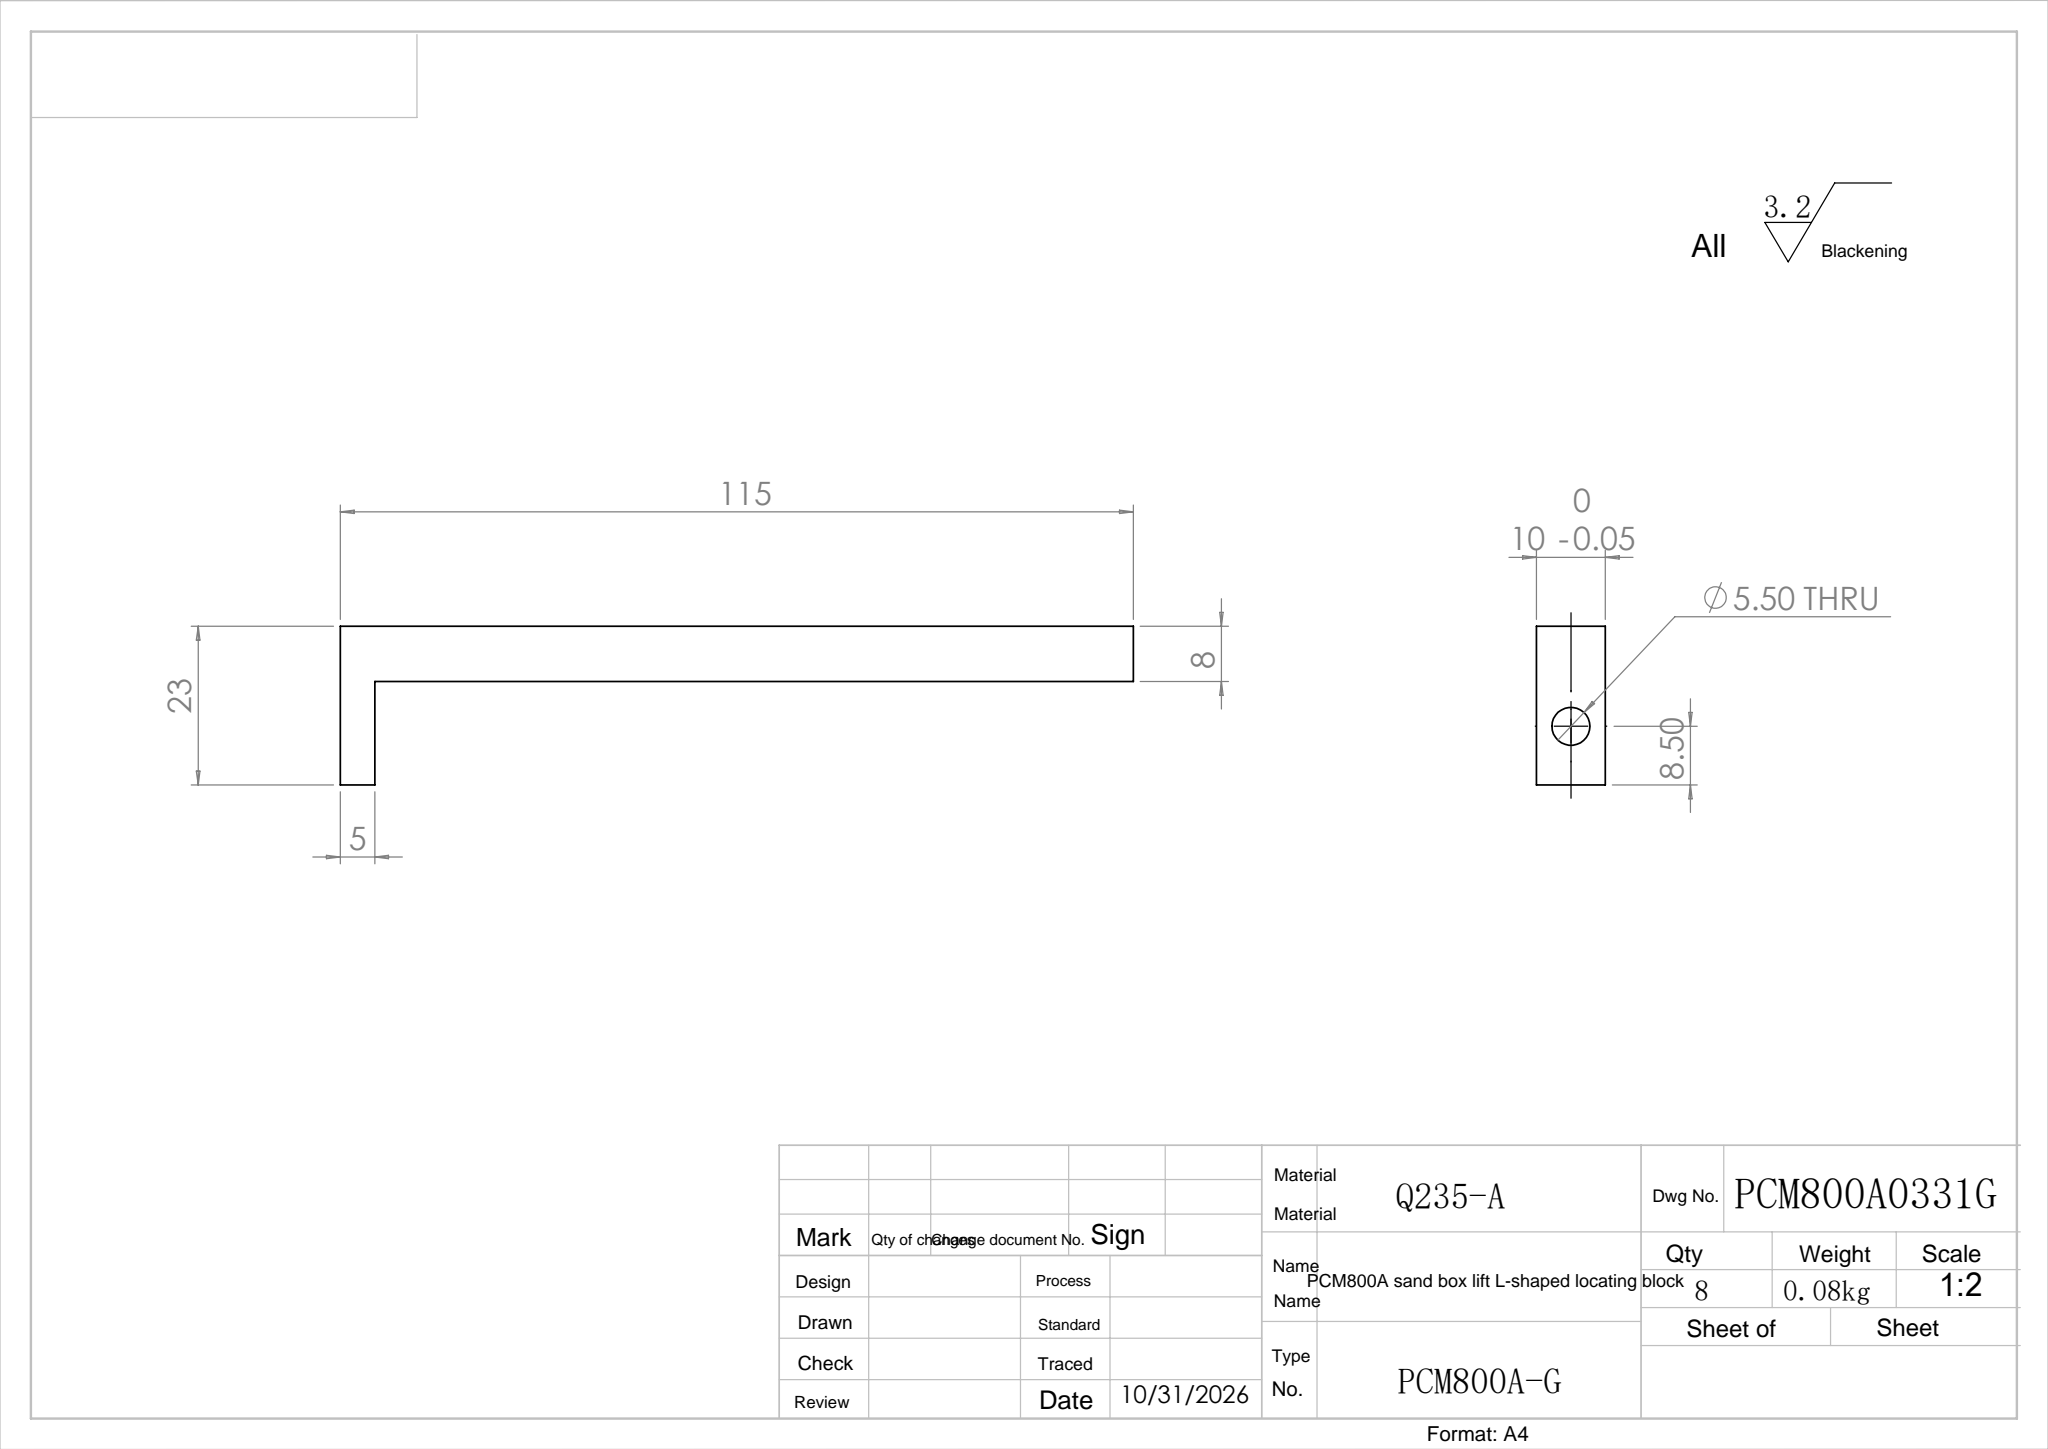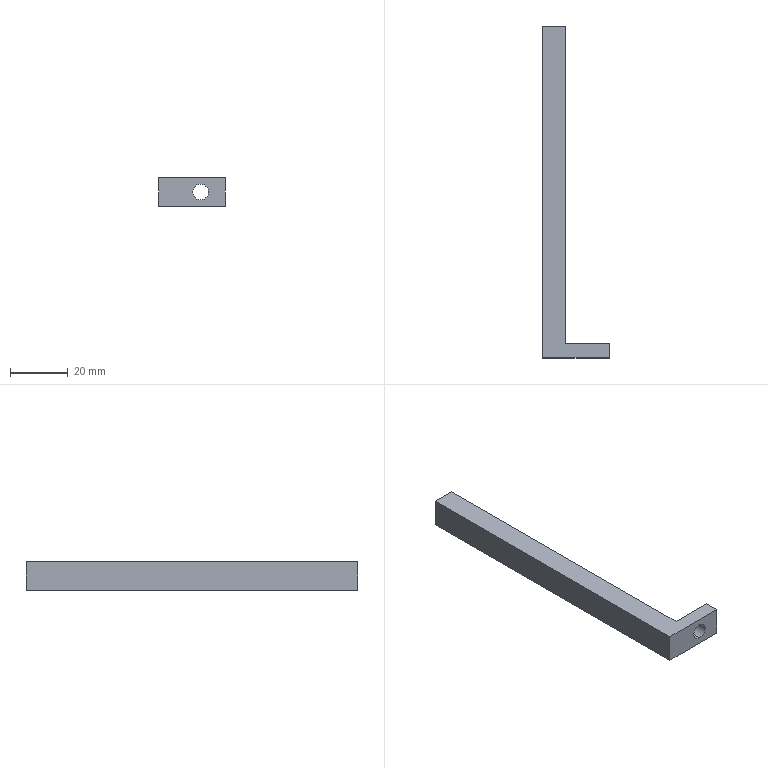Part | SolidWorks | features Extrusion 1, ICE 1 | 1 solid | 10 faces | box 23 x 115 x 10 mm | volume 9831 mm3 | plane 8 | cylinder 2 | commonest cylinder face diameters 5.5 x2
STEP:
#1=CARTESIAN_POINT('',(6.5,-110.,2.25));
#2=VERTEX_POINT('',#1);
#3=CARTESIAN_POINT('',(6.5,-110.,7.75));
#4=VERTEX_POINT('',#3);
#5=CARTESIAN_POINT('',(6.5,-110.,5.));
#6=DIRECTION('',(0.,1.,0.));
#7=DIRECTION('',(0.,0.,1.));
#8=AXIS2_PLACEMENT_3D('',#5,#6,#7);
#9=CIRCLE('',#8,2.75);
#10=EDGE_CURVE('',#2,#4,#9,.T.);
#11=ORIENTED_EDGE('',*,*,#10,.T.);
#12=CARTESIAN_POINT('',(6.5,-115.,7.75));
#13=VERTEX_POINT('',#12);
#14=CARTESIAN_POINT('',(6.5,0.,7.75));
#15=DIRECTION('',(0.,-1.,0.));
#16=VECTOR('',#15,1000.);
#17=LINE('',#14,#16);
#18=EDGE_CURVE('',#4,#13,#17,.T.);
#19=ORIENTED_EDGE('',*,*,#18,.T.);
#20=CARTESIAN_POINT('',(6.5,-115.,2.25));
#21=VERTEX_POINT('',#20);
#22=CARTESIAN_POINT('',(6.5,-115.,5.));
#23=DIRECTION('',(0.,-1.,0.));
#24=DIRECTION('',(0.,0.,-1.));
#25=AXIS2_PLACEMENT_3D('',#22,#23,#24);
#26=CIRCLE('',#25,2.75);
#27=EDGE_CURVE('',#13,#21,#26,.T.);
#28=ORIENTED_EDGE('',*,*,#27,.T.);
#29=CARTESIAN_POINT('',(6.5,0.,2.25));
#30=DIRECTION('',(0.,-1.,0.));
#31=VECTOR('',#30,1000.);
#32=LINE('',#29,#31);
#33=EDGE_CURVE('',#2,#21,#32,.T.);
#34=ORIENTED_EDGE('',*,*,#33,.F.);
#35=EDGE_LOOP('',(#11,#19,#28,#34));
#36=FACE_OUTER_BOUND('',#35,.T.);
#37=CARTESIAN_POINT('',(6.5,0.,5.));
#38=DIRECTION('',(0.,-1.,0.));
#39=DIRECTION('',(0.,0.,-1.));
#40=AXIS2_PLACEMENT_3D('',#37,#38,#39);
#41=CYLINDRICAL_SURFACE('',#40,2.75);
#42=ADVANCED_FACE('',(#36),#41,.F.);
#43=CARTESIAN_POINT('',(6.5,-115.,5.));
#44=DIRECTION('',(0.,-1.,0.));
#45=DIRECTION('',(0.,0.,-1.));
#46=AXIS2_PLACEMENT_3D('',#43,#44,#45);
#47=CIRCLE('',#46,2.75);
#48=EDGE_CURVE('',#21,#13,#47,.T.);
#49=ORIENTED_EDGE('',*,*,#48,.F.);
#50=ORIENTED_EDGE('',*,*,#27,.F.);
#51=EDGE_LOOP('',(#49,#50));
#52=FACE_BOUND('',#51,.T.);
#53=CARTESIAN_POINT('',(15.,-115.,0.));
#54=VERTEX_POINT('',#53);
#55=CARTESIAN_POINT('',(-8.,-115.,0.));
#56=VERTEX_POINT('',#55);
#57=CARTESIAN_POINT('',(3.5,-115.,0.));
#58=DIRECTION('',(-1.,0.,0.));
#59=VECTOR('',#58,1000.);
#60=LINE('',#57,#59);
#61=EDGE_CURVE('',#54,#56,#60,.T.);
#62=ORIENTED_EDGE('',*,*,#61,.F.);
#63=CARTESIAN_POINT('',(15.,-115.,10.));
#64=VERTEX_POINT('',#63);
#65=CARTESIAN_POINT('',(15.,-115.,10.));
#66=DIRECTION('',(0.,0.,-1.));
#67=VECTOR('',#66,1000.);
#68=LINE('',#65,#67);
#69=EDGE_CURVE('',#64,#54,#68,.T.);
#70=ORIENTED_EDGE('',*,*,#69,.F.);
#71=CARTESIAN_POINT('',(-8.,-115.,10.));
#72=VERTEX_POINT('',#71);
#73=CARTESIAN_POINT('',(3.5,-115.,10.));
#74=DIRECTION('',(-1.,0.,0.));
#75=VECTOR('',#74,1000.);
#76=LINE('',#73,#75);
#77=EDGE_CURVE('',#64,#72,#76,.T.);
#78=ORIENTED_EDGE('',*,*,#77,.T.);
#79=CARTESIAN_POINT('',(-8.,-115.,10.));
#80=DIRECTION('',(0.,0.,-1.));
#81=VECTOR('',#80,1000.);
#82=LINE('',#79,#81);
#83=EDGE_CURVE('',#72,#56,#82,.T.);
#84=ORIENTED_EDGE('',*,*,#83,.T.);
#85=EDGE_LOOP('',(#62,#70,#78,#84));
#86=FACE_OUTER_BOUND('',#85,.T.);
#87=CARTESIAN_POINT('',(3.5,-115.,10.));
#88=DIRECTION('',(0.,-1.,0.));
#89=DIRECTION('',(0.,0.,-1.));
#90=AXIS2_PLACEMENT_3D('',#87,#88,#89);
#91=PLANE('',#90);
#92=ADVANCED_FACE('',(#52,#86),#91,.T.);
#93=CARTESIAN_POINT('',(15.,-110.,0.));
#94=VERTEX_POINT('',#93);
#95=CARTESIAN_POINT('',(15.,-148.862,0.));
#96=DIRECTION('',(0.,-1.,0.));
#97=VECTOR('',#96,1000.);
#98=LINE('',#95,#97);
#99=EDGE_CURVE('',#94,#54,#98,.T.);
#100=ORIENTED_EDGE('',*,*,#99,.F.);
#101=CARTESIAN_POINT('',(15.,-110.,10.));
#102=VERTEX_POINT('',#101);
#103=CARTESIAN_POINT('',(15.,-110.,10.));
#104=DIRECTION('',(0.,0.,-1.));
#105=VECTOR('',#104,1000.);
#106=LINE('',#103,#105);
#107=EDGE_CURVE('',#102,#94,#106,.T.);
#108=ORIENTED_EDGE('',*,*,#107,.F.);
#109=CARTESIAN_POINT('',(15.,-148.862,10.));
#110=DIRECTION('',(0.,-1.,0.));
#111=VECTOR('',#110,1000.);
#112=LINE('',#109,#111);
#113=EDGE_CURVE('',#102,#64,#112,.T.);
#114=ORIENTED_EDGE('',*,*,#113,.T.);
#115=ORIENTED_EDGE('',*,*,#69,.T.);
#116=EDGE_LOOP('',(#100,#108,#114,#115));
#117=FACE_OUTER_BOUND('',#116,.T.);
#118=CARTESIAN_POINT('',(15.,-148.862,10.));
#119=DIRECTION('',(1.,0.,0.));
#120=DIRECTION('',(0.,0.,-1.));
#121=AXIS2_PLACEMENT_3D('',#118,#119,#120);
#122=PLANE('',#121);
#123=ADVANCED_FACE('',(#117),#122,.T.);
#124=ORIENTED_EDGE('',*,*,#10,.F.);
#125=CARTESIAN_POINT('',(6.5,-110.,5.));
#126=DIRECTION('',(0.,1.,0.));
#127=DIRECTION('',(0.,0.,1.));
#128=AXIS2_PLACEMENT_3D('',#125,#126,#127);
#129=CIRCLE('',#128,2.75);
#130=EDGE_CURVE('',#4,#2,#129,.T.);
#131=ORIENTED_EDGE('',*,*,#130,.F.);
#132=EDGE_LOOP('',(#124,#131));
#133=FACE_BOUND('',#132,.T.);
#134=CARTESIAN_POINT('',(0.,-110.,0.));
#135=VERTEX_POINT('',#134);
#136=CARTESIAN_POINT('',(3.5,-110.,0.));
#137=DIRECTION('',(1.,0.,0.));
#138=VECTOR('',#137,1000.);
#139=LINE('',#136,#138);
#140=EDGE_CURVE('',#135,#94,#139,.T.);
#141=ORIENTED_EDGE('',*,*,#140,.F.);
#142=CARTESIAN_POINT('',(0.,-110.,10.));
#143=VERTEX_POINT('',#142);
#144=CARTESIAN_POINT('',(0.,-110.,10.));
#145=DIRECTION('',(0.,0.,-1.));
#146=VECTOR('',#145,1000.);
#147=LINE('',#144,#146);
#148=EDGE_CURVE('',#143,#135,#147,.T.);
#149=ORIENTED_EDGE('',*,*,#148,.F.);
#150=CARTESIAN_POINT('',(3.5,-110.,10.));
#151=DIRECTION('',(1.,0.,0.));
#152=VECTOR('',#151,1000.);
#153=LINE('',#150,#152);
#154=EDGE_CURVE('',#143,#102,#153,.T.);
#155=ORIENTED_EDGE('',*,*,#154,.T.);
#156=ORIENTED_EDGE('',*,*,#107,.T.);
#157=EDGE_LOOP('',(#141,#149,#155,#156));
#158=FACE_OUTER_BOUND('',#157,.T.);
#159=CARTESIAN_POINT('',(3.5,-110.,10.));
#160=DIRECTION('',(0.,1.,0.));
#161=DIRECTION('',(0.,0.,1.));
#162=AXIS2_PLACEMENT_3D('',#159,#160,#161);
#163=PLANE('',#162);
#164=ADVANCED_FACE('',(#133,#158),#163,.T.);
#165=CARTESIAN_POINT('',(0.,0.,0.));
#166=VERTEX_POINT('',#165);
#167=CARTESIAN_POINT('',(0.,-148.862,0.));
#168=DIRECTION('',(0.,-1.,0.));
#169=VECTOR('',#168,1000.);
#170=LINE('',#167,#169);
#171=EDGE_CURVE('',#166,#135,#170,.T.);
#172=ORIENTED_EDGE('',*,*,#171,.F.);
#173=CARTESIAN_POINT('',(0.,0.,10.));
#174=VERTEX_POINT('',#173);
#175=CARTESIAN_POINT('',(0.,0.,10.));
#176=DIRECTION('',(0.,0.,-1.));
#177=VECTOR('',#176,1000.);
#178=LINE('',#175,#177);
#179=EDGE_CURVE('',#174,#166,#178,.T.);
#180=ORIENTED_EDGE('',*,*,#179,.F.);
#181=CARTESIAN_POINT('',(0.,-148.862,10.));
#182=DIRECTION('',(0.,-1.,0.));
#183=VECTOR('',#182,1000.);
#184=LINE('',#181,#183);
#185=EDGE_CURVE('',#174,#143,#184,.T.);
#186=ORIENTED_EDGE('',*,*,#185,.T.);
#187=ORIENTED_EDGE('',*,*,#148,.T.);
#188=EDGE_LOOP('',(#172,#180,#186,#187));
#189=FACE_OUTER_BOUND('',#188,.T.);
#190=CARTESIAN_POINT('',(0.,-148.862,10.));
#191=DIRECTION('',(1.,0.,0.));
#192=DIRECTION('',(0.,1.,0.));
#193=AXIS2_PLACEMENT_3D('',#190,#191,#192);
#194=PLANE('',#193);
#195=ADVANCED_FACE('',(#189),#194,.T.);
#196=CARTESIAN_POINT('',(-8.,0.,0.));
#197=VERTEX_POINT('',#196);
#198=CARTESIAN_POINT('',(3.5,0.,0.));
#199=DIRECTION('',(1.,0.,0.));
#200=VECTOR('',#199,1000.);
#201=LINE('',#198,#200);
#202=EDGE_CURVE('',#197,#166,#201,.T.);
#203=ORIENTED_EDGE('',*,*,#202,.F.);
#204=CARTESIAN_POINT('',(-8.,0.,10.));
#205=VERTEX_POINT('',#204);
#206=CARTESIAN_POINT('',(-8.,0.,10.));
#207=DIRECTION('',(0.,0.,-1.));
#208=VECTOR('',#207,1000.);
#209=LINE('',#206,#208);
#210=EDGE_CURVE('',#205,#197,#209,.T.);
#211=ORIENTED_EDGE('',*,*,#210,.F.);
#212=CARTESIAN_POINT('',(3.5,0.,10.));
#213=DIRECTION('',(1.,0.,0.));
#214=VECTOR('',#213,1000.);
#215=LINE('',#212,#214);
#216=EDGE_CURVE('',#205,#174,#215,.T.);
#217=ORIENTED_EDGE('',*,*,#216,.T.);
#218=ORIENTED_EDGE('',*,*,#179,.T.);
#219=EDGE_LOOP('',(#203,#211,#217,#218));
#220=FACE_OUTER_BOUND('',#219,.T.);
#221=CARTESIAN_POINT('',(3.5,0.,10.));
#222=DIRECTION('',(0.,1.,0.));
#223=DIRECTION('',(-1.,0.,0.));
#224=AXIS2_PLACEMENT_3D('',#221,#222,#223);
#225=PLANE('',#224);
#226=ADVANCED_FACE('',(#220),#225,.T.);
#227=CARTESIAN_POINT('',(-8.,-148.862,0.));
#228=DIRECTION('',(0.,-1.,0.));
#229=VECTOR('',#228,1000.);
#230=LINE('',#227,#229);
#231=EDGE_CURVE('',#197,#56,#230,.T.);
#232=ORIENTED_EDGE('',*,*,#231,.T.);
#233=ORIENTED_EDGE('',*,*,#83,.F.);
#234=CARTESIAN_POINT('',(-8.,-148.862,10.));
#235=DIRECTION('',(0.,-1.,0.));
#236=VECTOR('',#235,1000.);
#237=LINE('',#234,#236);
#238=EDGE_CURVE('',#205,#72,#237,.T.);
#239=ORIENTED_EDGE('',*,*,#238,.F.);
#240=ORIENTED_EDGE('',*,*,#210,.T.);
#241=EDGE_LOOP('',(#232,#233,#239,#240));
#242=FACE_OUTER_BOUND('',#241,.T.);
#243=CARTESIAN_POINT('',(-8.,-148.862,10.));
#244=DIRECTION('',(1.,0.,0.));
#245=DIRECTION('',(0.,1.,0.));
#246=AXIS2_PLACEMENT_3D('',#243,#244,#245);
#247=PLANE('',#246);
#248=ADVANCED_FACE('',(#242),#247,.F.);
#249=ORIENTED_EDGE('',*,*,#77,.F.);
#250=ORIENTED_EDGE('',*,*,#113,.F.);
#251=ORIENTED_EDGE('',*,*,#154,.F.);
#252=ORIENTED_EDGE('',*,*,#185,.F.);
#253=ORIENTED_EDGE('',*,*,#216,.F.);
#254=ORIENTED_EDGE('',*,*,#238,.T.);
#255=EDGE_LOOP('',(#249,#250,#251,#252,#253,#254));
#256=FACE_OUTER_BOUND('',#255,.T.);
#257=CARTESIAN_POINT('',(3.5,-148.862,10.));
#258=DIRECTION('',(0.,0.,1.));
#259=DIRECTION('',(1.,0.,0.));
#260=AXIS2_PLACEMENT_3D('',#257,#258,#259);
#261=PLANE('',#260);
#262=ADVANCED_FACE('',(#256),#261,.T.);
#263=ORIENTED_EDGE('',*,*,#61,.T.);
#264=ORIENTED_EDGE('',*,*,#231,.F.);
#265=ORIENTED_EDGE('',*,*,#202,.T.);
#266=ORIENTED_EDGE('',*,*,#171,.T.);
#267=ORIENTED_EDGE('',*,*,#140,.T.);
#268=ORIENTED_EDGE('',*,*,#99,.T.);
#269=EDGE_LOOP('',(#263,#264,#265,#266,#267,#268));
#270=FACE_OUTER_BOUND('',#269,.T.);
#271=CARTESIAN_POINT('',(3.5,-148.862,0.));
#272=DIRECTION('',(0.,0.,1.));
#273=DIRECTION('',(1.,0.,0.));
#274=AXIS2_PLACEMENT_3D('',#271,#272,#273);
#275=PLANE('',#274);
#276=ADVANCED_FACE('',(#270),#275,.F.);
#277=ORIENTED_EDGE('',*,*,#18,.F.);
#278=ORIENTED_EDGE('',*,*,#130,.T.);
#279=ORIENTED_EDGE('',*,*,#33,.T.);
#280=ORIENTED_EDGE('',*,*,#48,.T.);
#281=EDGE_LOOP('',(#277,#278,#279,#280));
#282=FACE_OUTER_BOUND('',#281,.T.);
#283=CARTESIAN_POINT('',(6.5,0.,5.));
#284=DIRECTION('',(0.,-1.,0.));
#285=DIRECTION('',(0.,0.,-1.));
#286=AXIS2_PLACEMENT_3D('',#283,#284,#285);
#287=CYLINDRICAL_SURFACE('',#286,2.75);
#288=ADVANCED_FACE('',(#282),#287,.F.);
#289=CLOSED_SHELL('',(#42,#92,#123,#164,#195,#226,#248,#262,#276,#288));
#290=MANIFOLD_SOLID_BREP('',#289);
#291=CARTESIAN_POINT('',(0.,0.,0.));
#292=DIRECTION('',(0.,0.,1.));
#293=DIRECTION('',(1.,0.,0.));
#294=AXIS2_PLACEMENT_3D('',#291,#292,#293);
#295=(LENGTH_UNIT()NAMED_UNIT(*)SI_UNIT(.MILLI.,.METRE.));
#296=UNCERTAINTY_MEASURE_WITH_UNIT(LENGTH_MEASURE(0.00001),#295,'','');
#297=(NAMED_UNIT(*)PLANE_ANGLE_UNIT()SI_UNIT($,.RADIAN.));
#298=(NAMED_UNIT(*)SI_UNIT($,.STERADIAN.)SOLID_ANGLE_UNIT());
#299=(GEOMETRIC_REPRESENTATION_CONTEXT(3)GLOBAL_UNCERTAINTY_ASSIGNED_CONTEXT((#296))GLOBAL_UNIT_ASSIGNED_CONTEXT((#295,#297,#298))REPRESENTATION_CONTEXT('',''));
#300=ADVANCED_BREP_SHAPE_REPRESENTATION('',(#290,#294),#299);